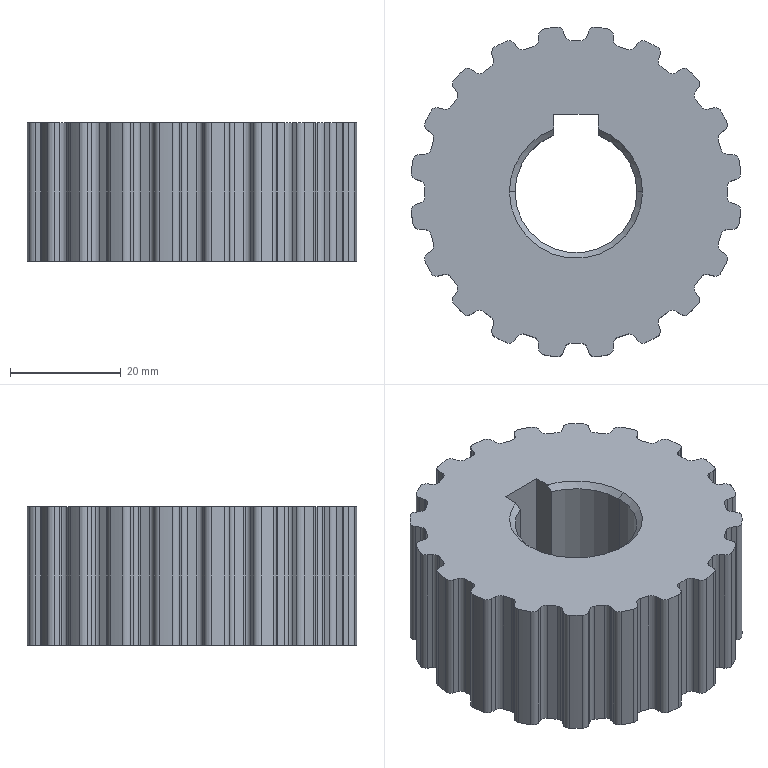Part | STEP file | Small pulley | 1 solid | 186 faces | box 59.476 x 59.476 x 25 mm | volume 54452 mm3 | cylinder 117 | plane 65 | cone 4 | commonest cylinder face diameters 2.34 x48 2.38 x46 59.88 x20 22 x3